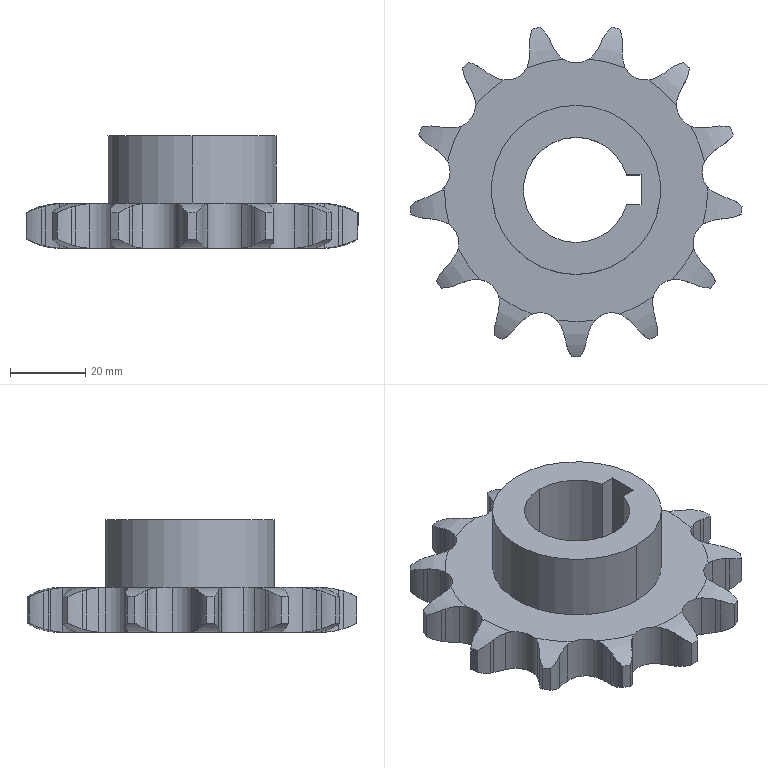Part | SolidWorks | features BaseBody 1 | 1 solid | 150 faces | box 88.308 x 87.678 x 30 mm | volume 62261 mm3 | cylinder 90 | plane 32 | spline 28 | commonest cylinder face diameters 20.039 x28 31.085 x27 12.029 x17 88.719 x13 28 x3 45 x2